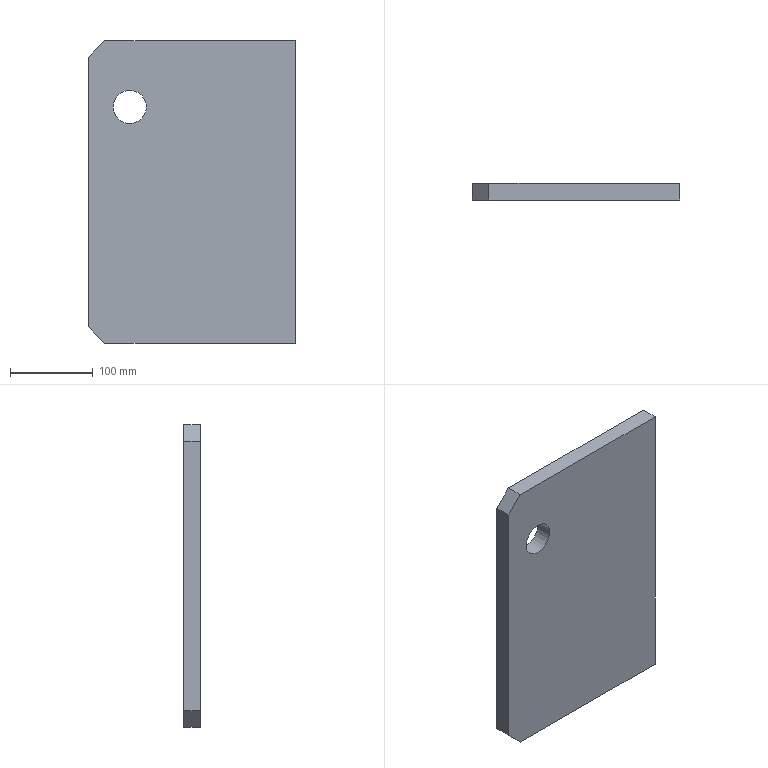Part | SolidWorks | features Chamfer 2, Extrusion 1, ICE 1 | 1 solid | 10 faces | box 250 x 20 x 365 mm | volume 1791867 mm3 | plane 8 | cylinder 2 | commonest cylinder face diameters 40 x2
STEP:
#1=CARTESIAN_POINT('',(-180.,0.,285.));
#2=VERTEX_POINT('',#1);
#3=CARTESIAN_POINT('',(-220.,0.,285.));
#4=VERTEX_POINT('',#3);
#5=CARTESIAN_POINT('',(-200.,0.,285.));
#6=DIRECTION('',(0.,1.,0.));
#7=DIRECTION('',(-1.,0.,0.));
#8=AXIS2_PLACEMENT_3D('',#5,#6,#7);
#9=CIRCLE('',#8,20.);
#10=EDGE_CURVE('',#2,#4,#9,.T.);
#11=ORIENTED_EDGE('',*,*,#10,.F.);
#12=CARTESIAN_POINT('',(-180.,20.,285.));
#13=VERTEX_POINT('',#12);
#14=CARTESIAN_POINT('',(-180.,0.,285.));
#15=DIRECTION('',(0.,1.,0.));
#16=VECTOR('',#15,1000.);
#17=LINE('',#14,#16);
#18=EDGE_CURVE('',#2,#13,#17,.T.);
#19=ORIENTED_EDGE('',*,*,#18,.T.);
#20=CARTESIAN_POINT('',(-220.,20.,285.));
#21=VERTEX_POINT('',#20);
#22=CARTESIAN_POINT('',(-200.,20.,285.));
#23=DIRECTION('',(0.,-1.,0.));
#24=DIRECTION('',(1.,0.,0.));
#25=AXIS2_PLACEMENT_3D('',#22,#23,#24);
#26=CIRCLE('',#25,20.);
#27=EDGE_CURVE('',#21,#13,#26,.T.);
#28=ORIENTED_EDGE('',*,*,#27,.F.);
#29=CARTESIAN_POINT('',(-220.,0.,285.));
#30=DIRECTION('',(0.,1.,0.));
#31=VECTOR('',#30,1000.);
#32=LINE('',#29,#31);
#33=EDGE_CURVE('',#4,#21,#32,.T.);
#34=ORIENTED_EDGE('',*,*,#33,.F.);
#35=EDGE_LOOP('',(#11,#19,#28,#34));
#36=FACE_OUTER_BOUND('',#35,.T.);
#37=CARTESIAN_POINT('',(-200.,0.,285.));
#38=DIRECTION('',(0.,1.,0.));
#39=DIRECTION('',(-1.,0.,0.));
#40=AXIS2_PLACEMENT_3D('',#37,#38,#39);
#41=CYLINDRICAL_SURFACE('',#40,20.);
#42=ADVANCED_FACE('',(#36),#41,.F.);
#43=CARTESIAN_POINT('',(0.,0.,0.));
#44=VERTEX_POINT('',#43);
#45=CARTESIAN_POINT('',(0.,20.,0.));
#46=VERTEX_POINT('',#45);
#47=CARTESIAN_POINT('',(0.,0.,0.));
#48=DIRECTION('',(0.,1.,0.));
#49=VECTOR('',#48,1000.);
#50=LINE('',#47,#49);
#51=EDGE_CURVE('',#44,#46,#50,.T.);
#52=ORIENTED_EDGE('',*,*,#51,.T.);
#53=CARTESIAN_POINT('',(0.,20.,365.));
#54=VERTEX_POINT('',#53);
#55=CARTESIAN_POINT('',(0.,20.,365.));
#56=DIRECTION('',(0.,0.,-1.));
#57=VECTOR('',#56,1000.);
#58=LINE('',#55,#57);
#59=EDGE_CURVE('',#54,#46,#58,.T.);
#60=ORIENTED_EDGE('',*,*,#59,.F.);
#61=CARTESIAN_POINT('',(0.,0.,365.));
#62=VERTEX_POINT('',#61);
#63=CARTESIAN_POINT('',(0.,0.,365.));
#64=DIRECTION('',(0.,1.,0.));
#65=VECTOR('',#64,1000.);
#66=LINE('',#63,#65);
#67=EDGE_CURVE('',#62,#54,#66,.T.);
#68=ORIENTED_EDGE('',*,*,#67,.F.);
#69=CARTESIAN_POINT('',(0.,0.,365.));
#70=DIRECTION('',(0.,0.,-1.));
#71=VECTOR('',#70,1000.);
#72=LINE('',#69,#71);
#73=EDGE_CURVE('',#62,#44,#72,.T.);
#74=ORIENTED_EDGE('',*,*,#73,.T.);
#75=EDGE_LOOP('',(#52,#60,#68,#74));
#76=FACE_OUTER_BOUND('',#75,.T.);
#77=CARTESIAN_POINT('',(0.,0.,365.));
#78=DIRECTION('',(-1.,0.,0.));
#79=DIRECTION('',(0.,-1.,0.));
#80=AXIS2_PLACEMENT_3D('',#77,#78,#79);
#81=PLANE('',#80);
#82=ADVANCED_FACE('',(#76),#81,.F.);
#83=ORIENTED_EDGE('',*,*,#27,.T.);
#84=CARTESIAN_POINT('',(-200.,20.,285.));
#85=DIRECTION('',(0.,-1.,0.));
#86=DIRECTION('',(1.,0.,0.));
#87=AXIS2_PLACEMENT_3D('',#84,#85,#86);
#88=CIRCLE('',#87,20.);
#89=EDGE_CURVE('',#13,#21,#88,.T.);
#90=ORIENTED_EDGE('',*,*,#89,.T.);
#91=EDGE_LOOP('',(#83,#90));
#92=FACE_BOUND('',#91,.T.);
#93=CARTESIAN_POINT('',(-230.,20.,0.));
#94=VERTEX_POINT('',#93);
#95=CARTESIAN_POINT('',(0.,20.,0.));
#96=DIRECTION('',(-1.,0.,0.));
#97=VECTOR('',#96,1000.);
#98=LINE('',#95,#97);
#99=EDGE_CURVE('',#46,#94,#98,.T.);
#100=ORIENTED_EDGE('',*,*,#99,.T.);
#101=CARTESIAN_POINT('',(-250.,20.,20.));
#102=VERTEX_POINT('',#101);
#103=CARTESIAN_POINT('',(-250.,20.,20.));
#104=DIRECTION('',(-0.7071,0.,0.7071));
#105=VECTOR('',#104,1000.);
#106=LINE('',#103,#105);
#107=EDGE_CURVE('',#94,#102,#106,.T.);
#108=ORIENTED_EDGE('',*,*,#107,.T.);
#109=CARTESIAN_POINT('',(-250.,20.,345.));
#110=VERTEX_POINT('',#109);
#111=CARTESIAN_POINT('',(-250.,20.,365.));
#112=DIRECTION('',(0.,0.,-1.));
#113=VECTOR('',#112,1000.);
#114=LINE('',#111,#113);
#115=EDGE_CURVE('',#110,#102,#114,.T.);
#116=ORIENTED_EDGE('',*,*,#115,.F.);
#117=CARTESIAN_POINT('',(-230.,20.,365.));
#118=VERTEX_POINT('',#117);
#119=CARTESIAN_POINT('',(-230.,20.,365.));
#120=DIRECTION('',(0.7071,0.,0.7071));
#121=VECTOR('',#120,1000.);
#122=LINE('',#119,#121);
#123=EDGE_CURVE('',#110,#118,#122,.T.);
#124=ORIENTED_EDGE('',*,*,#123,.T.);
#125=CARTESIAN_POINT('',(0.,20.,365.));
#126=DIRECTION('',(-1.,0.,0.));
#127=VECTOR('',#126,1000.);
#128=LINE('',#125,#127);
#129=EDGE_CURVE('',#54,#118,#128,.T.);
#130=ORIENTED_EDGE('',*,*,#129,.F.);
#131=ORIENTED_EDGE('',*,*,#59,.T.);
#132=EDGE_LOOP('',(#100,#108,#116,#124,#130,#131));
#133=FACE_OUTER_BOUND('',#132,.T.);
#134=CARTESIAN_POINT('',(0.,20.,365.));
#135=DIRECTION('',(0.,-1.,0.));
#136=DIRECTION('',(1.,0.,0.));
#137=AXIS2_PLACEMENT_3D('',#134,#135,#136);
#138=PLANE('',#137);
#139=ADVANCED_FACE('',(#92,#133),#138,.F.);
#140=ORIENTED_EDGE('',*,*,#115,.T.);
#141=CARTESIAN_POINT('',(-250.,0.,20.));
#142=VERTEX_POINT('',#141);
#143=CARTESIAN_POINT('',(-250.,0.,20.));
#144=DIRECTION('',(0.,-1.,0.));
#145=VECTOR('',#144,1000.);
#146=LINE('',#143,#145);
#147=EDGE_CURVE('',#102,#142,#146,.T.);
#148=ORIENTED_EDGE('',*,*,#147,.T.);
#149=CARTESIAN_POINT('',(-250.,0.,345.));
#150=VERTEX_POINT('',#149);
#151=CARTESIAN_POINT('',(-250.,0.,365.));
#152=DIRECTION('',(0.,0.,-1.));
#153=VECTOR('',#152,1000.);
#154=LINE('',#151,#153);
#155=EDGE_CURVE('',#150,#142,#154,.T.);
#156=ORIENTED_EDGE('',*,*,#155,.F.);
#157=CARTESIAN_POINT('',(-250.,20.,345.));
#158=DIRECTION('',(0.,1.,0.));
#159=VECTOR('',#158,1000.);
#160=LINE('',#157,#159);
#161=EDGE_CURVE('',#150,#110,#160,.T.);
#162=ORIENTED_EDGE('',*,*,#161,.T.);
#163=EDGE_LOOP('',(#140,#148,#156,#162));
#164=FACE_OUTER_BOUND('',#163,.T.);
#165=CARTESIAN_POINT('',(-250.,0.,365.));
#166=DIRECTION('',(1.,0.,0.));
#167=DIRECTION('',(0.,0.,-1.));
#168=AXIS2_PLACEMENT_3D('',#165,#166,#167);
#169=PLANE('',#168);
#170=ADVANCED_FACE('',(#164),#169,.F.);
#171=CARTESIAN_POINT('',(-200.,0.,285.));
#172=DIRECTION('',(0.,1.,0.));
#173=DIRECTION('',(-1.,0.,0.));
#174=AXIS2_PLACEMENT_3D('',#171,#172,#173);
#175=CIRCLE('',#174,20.);
#176=EDGE_CURVE('',#4,#2,#175,.T.);
#177=ORIENTED_EDGE('',*,*,#176,.T.);
#178=ORIENTED_EDGE('',*,*,#10,.T.);
#179=EDGE_LOOP('',(#177,#178));
#180=FACE_BOUND('',#179,.T.);
#181=ORIENTED_EDGE('',*,*,#155,.T.);
#182=CARTESIAN_POINT('',(-230.,0.,0.));
#183=VERTEX_POINT('',#182);
#184=CARTESIAN_POINT('',(-250.,0.,20.));
#185=DIRECTION('',(0.7071,0.,-0.7071));
#186=VECTOR('',#185,1000.);
#187=LINE('',#184,#186);
#188=EDGE_CURVE('',#142,#183,#187,.T.);
#189=ORIENTED_EDGE('',*,*,#188,.T.);
#190=CARTESIAN_POINT('',(0.,0.,0.));
#191=DIRECTION('',(1.,0.,0.));
#192=VECTOR('',#191,1000.);
#193=LINE('',#190,#192);
#194=EDGE_CURVE('',#183,#44,#193,.T.);
#195=ORIENTED_EDGE('',*,*,#194,.T.);
#196=ORIENTED_EDGE('',*,*,#73,.F.);
#197=CARTESIAN_POINT('',(-230.,0.,365.));
#198=VERTEX_POINT('',#197);
#199=CARTESIAN_POINT('',(0.,0.,365.));
#200=DIRECTION('',(1.,0.,0.));
#201=VECTOR('',#200,1000.);
#202=LINE('',#199,#201);
#203=EDGE_CURVE('',#198,#62,#202,.T.);
#204=ORIENTED_EDGE('',*,*,#203,.F.);
#205=CARTESIAN_POINT('',(-230.,0.,365.));
#206=DIRECTION('',(-0.7071,0.,-0.7071));
#207=VECTOR('',#206,1000.);
#208=LINE('',#205,#207);
#209=EDGE_CURVE('',#198,#150,#208,.T.);
#210=ORIENTED_EDGE('',*,*,#209,.T.);
#211=EDGE_LOOP('',(#181,#189,#195,#196,#204,#210));
#212=FACE_OUTER_BOUND('',#211,.T.);
#213=CARTESIAN_POINT('',(0.,0.,365.));
#214=DIRECTION('',(0.,1.,0.));
#215=DIRECTION('',(0.,0.,1.));
#216=AXIS2_PLACEMENT_3D('',#213,#214,#215);
#217=PLANE('',#216);
#218=ADVANCED_FACE('',(#180,#212),#217,.F.);
#219=ORIENTED_EDGE('',*,*,#129,.T.);
#220=CARTESIAN_POINT('',(-230.,0.,365.));
#221=DIRECTION('',(0.,-1.,0.));
#222=VECTOR('',#221,1000.);
#223=LINE('',#220,#222);
#224=EDGE_CURVE('',#118,#198,#223,.T.);
#225=ORIENTED_EDGE('',*,*,#224,.T.);
#226=ORIENTED_EDGE('',*,*,#203,.T.);
#227=ORIENTED_EDGE('',*,*,#67,.T.);
#228=EDGE_LOOP('',(#219,#225,#226,#227));
#229=FACE_OUTER_BOUND('',#228,.T.);
#230=CARTESIAN_POINT('',(0.,0.,365.));
#231=DIRECTION('',(0.,0.,1.));
#232=DIRECTION('',(1.,0.,0.));
#233=AXIS2_PLACEMENT_3D('',#230,#231,#232);
#234=PLANE('',#233);
#235=ADVANCED_FACE('',(#229),#234,.T.);
#236=ORIENTED_EDGE('',*,*,#194,.F.);
#237=CARTESIAN_POINT('',(-230.,0.,0.));
#238=DIRECTION('',(0.,1.,0.));
#239=VECTOR('',#238,1000.);
#240=LINE('',#237,#239);
#241=EDGE_CURVE('',#183,#94,#240,.T.);
#242=ORIENTED_EDGE('',*,*,#241,.T.);
#243=ORIENTED_EDGE('',*,*,#99,.F.);
#244=ORIENTED_EDGE('',*,*,#51,.F.);
#245=EDGE_LOOP('',(#236,#242,#243,#244));
#246=FACE_OUTER_BOUND('',#245,.T.);
#247=CARTESIAN_POINT('',(0.,0.,0.));
#248=DIRECTION('',(0.,0.,1.));
#249=DIRECTION('',(1.,0.,0.));
#250=AXIS2_PLACEMENT_3D('',#247,#248,#249);
#251=PLANE('',#250);
#252=ADVANCED_FACE('',(#246),#251,.F.);
#253=ORIENTED_EDGE('',*,*,#123,.F.);
#254=ORIENTED_EDGE('',*,*,#161,.F.);
#255=ORIENTED_EDGE('',*,*,#209,.F.);
#256=ORIENTED_EDGE('',*,*,#224,.F.);
#257=EDGE_LOOP('',(#253,#254,#255,#256));
#258=FACE_OUTER_BOUND('',#257,.T.);
#259=CARTESIAN_POINT('',(-230.,0.,365.));
#260=DIRECTION('',(-0.7071,0.,0.7071));
#261=DIRECTION('',(0.,1.,0.));
#262=AXIS2_PLACEMENT_3D('',#259,#260,#261);
#263=PLANE('',#262);
#264=ADVANCED_FACE('',(#258),#263,.T.);
#265=ORIENTED_EDGE('',*,*,#18,.F.);
#266=ORIENTED_EDGE('',*,*,#176,.F.);
#267=ORIENTED_EDGE('',*,*,#33,.T.);
#268=ORIENTED_EDGE('',*,*,#89,.F.);
#269=EDGE_LOOP('',(#265,#266,#267,#268));
#270=FACE_OUTER_BOUND('',#269,.T.);
#271=CARTESIAN_POINT('',(-200.,0.,285.));
#272=DIRECTION('',(0.,1.,0.));
#273=DIRECTION('',(-1.,0.,0.));
#274=AXIS2_PLACEMENT_3D('',#271,#272,#273);
#275=CYLINDRICAL_SURFACE('',#274,20.);
#276=ADVANCED_FACE('',(#270),#275,.F.);
#277=ORIENTED_EDGE('',*,*,#107,.F.);
#278=ORIENTED_EDGE('',*,*,#241,.F.);
#279=ORIENTED_EDGE('',*,*,#188,.F.);
#280=ORIENTED_EDGE('',*,*,#147,.F.);
#281=EDGE_LOOP('',(#277,#278,#279,#280));
#282=FACE_OUTER_BOUND('',#281,.T.);
#283=CARTESIAN_POINT('',(-250.,0.,20.));
#284=DIRECTION('',(0.7071,0.,0.7071));
#285=DIRECTION('',(0.,-1.,0.));
#286=AXIS2_PLACEMENT_3D('',#283,#284,#285);
#287=PLANE('',#286);
#288=ADVANCED_FACE('',(#282),#287,.F.);
#289=CLOSED_SHELL('',(#42,#82,#139,#170,#218,#235,#252,#264,#276,#288));
#290=MANIFOLD_SOLID_BREP('',#289);
#291=CARTESIAN_POINT('',(0.,0.,0.));
#292=DIRECTION('',(0.,0.,1.));
#293=DIRECTION('',(1.,0.,0.));
#294=AXIS2_PLACEMENT_3D('',#291,#292,#293);
#295=(LENGTH_UNIT()NAMED_UNIT(*)SI_UNIT(.MILLI.,.METRE.));
#296=UNCERTAINTY_MEASURE_WITH_UNIT(LENGTH_MEASURE(0.00001),#295,'','');
#297=(NAMED_UNIT(*)PLANE_ANGLE_UNIT()SI_UNIT($,.RADIAN.));
#298=(NAMED_UNIT(*)SI_UNIT($,.STERADIAN.)SOLID_ANGLE_UNIT());
#299=(GEOMETRIC_REPRESENTATION_CONTEXT(3)GLOBAL_UNCERTAINTY_ASSIGNED_CONTEXT((#296))GLOBAL_UNIT_ASSIGNED_CONTEXT((#295,#297,#298))REPRESENTATION_CONTEXT('',''));
#300=ADVANCED_BREP_SHAPE_REPRESENTATION('',(#290,#294),#299);